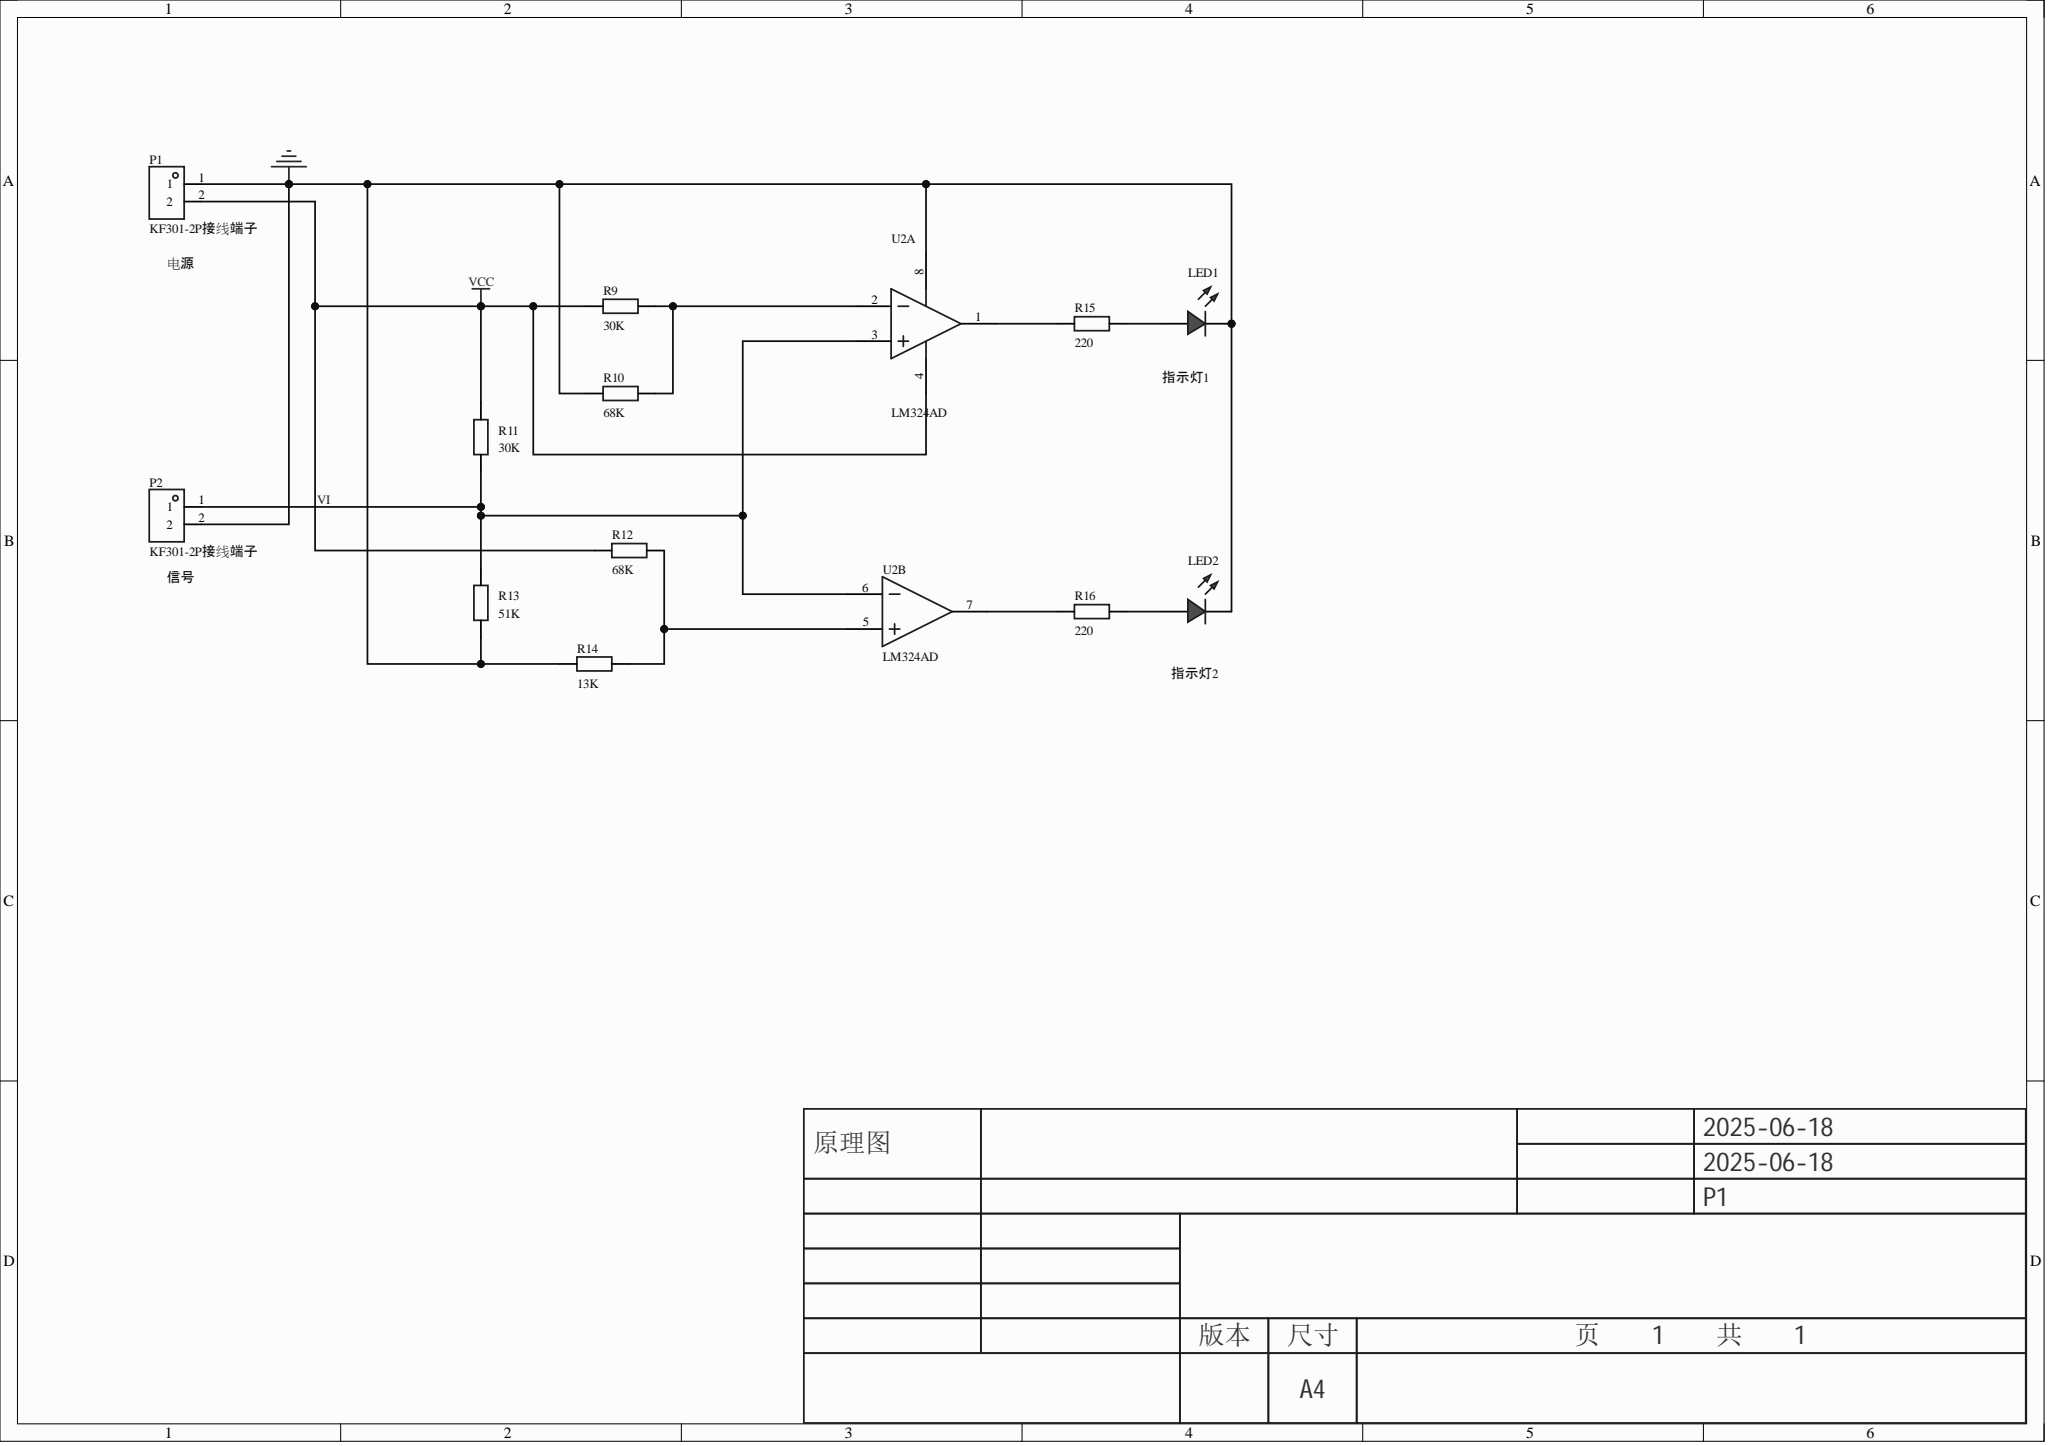Circuit board | Altium Designer | 13 parts | 9 nets
Bill of materials:
Comment,Description,Designator,Footprint,LibRef,Quantity
"","","LED1, LED2","LED_TH-3mm","LED_TH-R_3mm","2"
"KF301-2P接线端子","","P1, P2","CONN-TH_XY301V-A-5.0-2P","KF301-2P接线端子","2"
"30K","","R9, R11","Res_1/8W","Res_AXIAL-1/8W","2"
"68K","","R10, R12","Res_1/8W","Res_AXIAL-1/8W","2"
"51K","","R13","Res_1/8W","Res_AXIAL-1/8W","1"
"13K","","R14","Res_1/8W","Res_AXIAL-1/8W","1"
"220","","R15, R16","Res_1/8W","Res_AXIAL-1/8W","2"
"LM324AD","放大器数:双路;轨到轨:-;增益带宽积(GBP):10MHz;输入失调电压(Vos):5mV;压摆率(SR):11V/us;输入偏置电流(Ib):500nA;","U2","DIP-8_L9.3-W6.4-P2.54-LS7.6-BL","NE5532N","1"
Netlist (Protel format):
[
LED1
LED_TH-3mm




]
[
LED2
LED_TH-3mm




]
[
P1
CONN-TH_XY301V-A-5.0-2P
KF301-2P接线端子



]
[
P2
CONN-TH_XY301V-A-5.0-2P
KF301-2P接线端子



]
[
R9
Res_1/8W
30K



]
[
R10
Res_1/8W
68K



]
[
R11
Res_1/8W
30K



]
[
R12
Res_1/8W
68K



]
[
R13
Res_1/8W
51K



]
[
R14
Res_1/8W
13K



]
[
R15
Res_1/8W
220



]
[
R16
Res_1/8W
220



]
[
U2
DIP-8_L9.3-W6.4-P2.54-LS7.6-BL
LM324AD



]
(
VI
P2-1
R11-1
R13-2
U2-3
U2-6
)
(
VCC
P1-2
R9-1
R11-2
R12-1
U2-4
)
(
NetR16_1
R16-1
U2-7
)
(
NetR15_1
R15-1
U2-1
)
(
NetR12_2
R12-2
R14-2
U2-5
)
(
NetR9_2
R9-2
R10-2
U2-2
)
(
NetLED2_1
LED2-1
R16-2
)
(
NetLED1_1
LED1-1
R15-2
)
(
GND
LED1-2
LED2-2
P1-1
P2-2
R10-1
R13-1
R14-1
U2-8
)